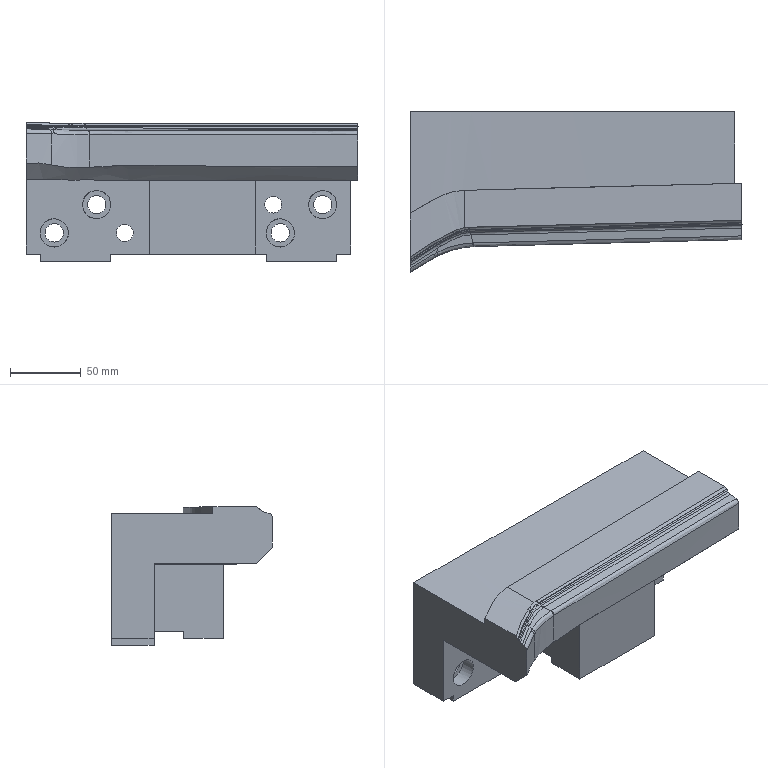Part | NX | features solid 2 | 1 solid | 73 faces | box 235 x 113.719 x 97.89 mm | volume 1324121 mm3 | spline 39 | plane 24 | cylinder 10 | commonest cylinder face diameters 13 x4 20 x4 12 x2